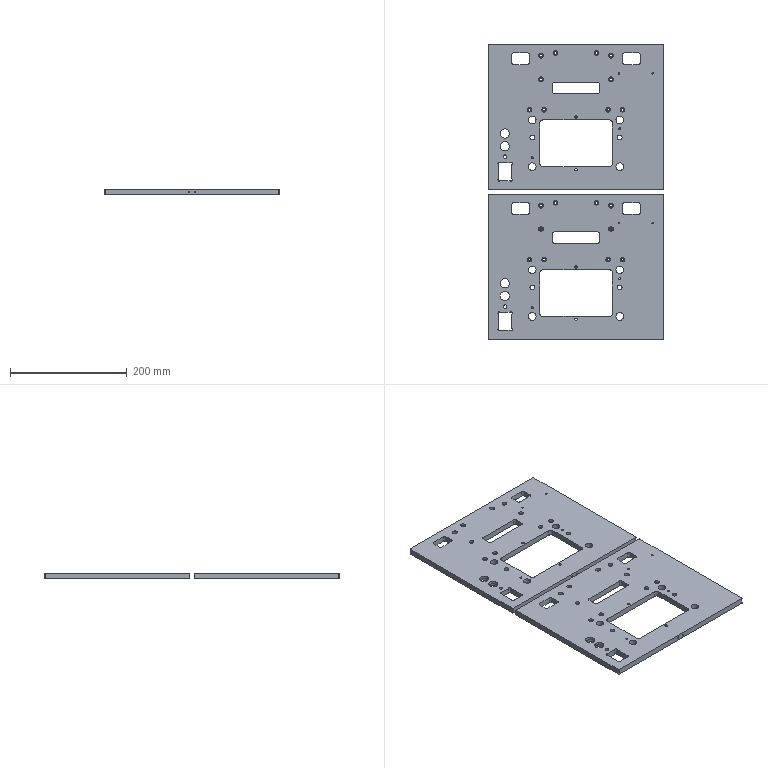NC program | NX | posted with a generic post | part box 300 x 507 x 10 mm
Whole program:
N10 G17 G21 G94 G90
(ZLEVEL_PROFILE_1_COPY_1_COPY_COPY , TOOL : D4A45)
N12 T02 M6
N14 G54
N16 G17 G0 G90 X44.225 Y79.686 S9500 M3
N18 G43 Z30. H2
N20 Z0.
N22 G94 G1 Z-1. F1000.
N24 X43.846 Y80.341
N26 G3 X43.5 Y80.541 R0.4
N28 X37.959 Y75. R5.541
N30 X43.5 Y80.541 R-5.541
N32 X43.154 Y80.341 R0.4
N34 G1 X42.775 Y79.686
N36 Z0.
N38 G0 Z30.
N40 X38.592 Y0.223
N42 Z0.
N44 G1 Z-1.
N46 X38.846 Y0.841
N48 G3 X38.5 Y1.041 R0.4
N50 X37.459 Y0. R1.041
N52 X38.5 Y1.041 R-1.041
N54 X38.154 Y0.841 R0.4
N56 G1 X38.408 Y0.223
N58 Z0.
N60 G0 Z30.
N62 X203.5 Y-131.791
N64 Z1.
N66 G1 Z-1.
N68 G3 X203.791 Y-131.5 R0.291
N70 X203.5 Y-131.791 R-0.291
N72 X203.673 Y-131.691 R0.2
N74 G1 Z0.
N76 G0 Z30.
N78 X48.178 Y131.357
N80 Z0.
N82 G1 Z-1.
N84 X47.898 Y131.841
N86 G3 X47.551 Y132.041 R0.4
N88 G1 X22.449
N90 G2 X21.694 Y132.41 R0.966
N92 G3 X20.094 Y130.803 R-1.141
N94 G2 X20.459 Y130.051 R0.956
N96 G1 Y112.949
N98 G2 X20.09 Y112.193 R0.967
N100 G3 X21.697 Y110.594 R-1.141
N102 G2 X22.449 Y110.959 R0.957
N104 G1 X47.551
N106 G2 X48.308 Y110.588 R0.97
N108 G3 X49.906 Y112.197 R-1.141
N110 G2 X49.541 Y112.949 R0.956
N112 G1 Y130.051
N114 G2 X49.911 Y130.807 R0.968
N116 G3 X48.303 Y132.406 R-1.141
N118 G2 X47.551 Y132.041 R0.957
N120 G3 X47.205 Y131.842 R0.4
N122 G1 X46.858 Y131.241
N124 Z0.
N126 G0 Z30.
N128 X140.228 Y-57.354
N130 Z0.
N132 G1 Z-1.
N134 X140.654 Y-58.091
N136 G3 X141. Y-58.291 R0.4
N138 G1 X141.001
N140 G3 X144.041 Y-55.249 R3.041
N142 X141. Y-58.291 R-3.041
N144 X141.346 Y-58.091 R0.4
N146 G1 X141.772 Y-57.354
N148 Z0.
N150 G0 Z30.
N152 X140.228 Y-82.104
N154 Z0.
N156 G1 Z-1.
N158 X140.654 Y-82.841
N160 G3 X141. Y-83.041 R0.4
N162 G1 X141.001
N164 G3 X144.041 Y-79.999 R3.041
N166 X141. Y-83.041 R-3.041
N168 X141.346 Y-82.841 R0.4
N170 G1 X141.772 Y-82.104
N172 Z0.
N174 G0 Z30.
N176 Y56.854
N178 Z0.
N180 G1 Z-1.
N182 X141.346 Y57.591
N184 G3 X141. Y57.791 R0.4
N186 X137.959 Y54.75 R3.041
N188 X141. Y57.791 R-3.041
N190 X140.654 Y57.591 R0.4
N192 G1 X140.228 Y56.854
N194 Z0.
N196 G0 Z30.
N198 X141.772 Y82.104
N200 Z0.
N202 G1 Z-1.
N204 X141.346 Y82.841
N206 G3 X141. Y83.041 R0.4
N208 X137.959 Y80. R3.041
N210 X141. Y83.041 R-3.041
N212 X140.654 Y82.841 R0.4
N214 G1 X140.228 Y82.104
N216 Z0.
N218 G0 Z30.
N220 X128.723 Y-0.092
N222 Z0.
N224 G1 Z-1.
N226 X129.341 Y-0.346
N228 G3 X129.541 Y0. R0.4
N230 X128.5 Y1.041 R1.041
N232 X129.541 Y0. R-1.041
N234 X129.341 Y0.346 R0.4
N236 G1 X128.723 Y0.092
N238 Z0.
N240 G0 Z30.
N242 X203.791 Y-73.5
N244 Z1.
N246 G1 Z-1.
N248 G3 X203.5 Y-73.209 R0.291
N250 X203.791 Y-73.5 R-0.291
N252 X203.691 Y-73.327 R0.2
N254 G1 Z0.
N256 G0 Z30.
N258 X235.604 Y-60.772
N260 Z0.
N262 G1 Z-1.
N264 X236.341 Y-60.346
N266 G3 X236.541 Y-60. R0.4
N268 X233.5 Y-56.959 R3.041
N270 X236.541 Y-60. R-3.041
N272 X236.341 Y-59.654 R0.4
N274 G1 X235.604 Y-59.228
N276 Z0.
N278 G0 Z30.
N280 X122.775 Y-79.686
N282 Z0.
N284 G1 Z-1.
N286 X123.154 Y-80.341
N288 G3 X123.5 Y-80.541 R0.4
N290 X129.041 Y-75. R5.541
N292 X123.5 Y-80.541 R-5.541
N294 X123.846 Y-80.341 R0.4
N296 G1 X124.225 Y-79.686
N298 Z0.
N300 G0 Z30.
N302 Y79.686
N304 Z0.
N306 G1 Z-1.
N308 X123.846 Y80.341
N310 G3 X123.5 Y80.541 R0.4
N312 G1 X123.496
N314 G3 X117.959 Y74.996 R5.541
N316 X123.5 Y80.541 R-5.541
N318 X123.154 Y80.341 R0.4
N320 G1 X122.775 Y79.686
N322 Z0.
N324 G0 Z30.
N326 X108.5 Y-75.691
N328 Z1.
N330 G1 Z-1.
N332 X108.501
N334 G3 X109.191 Y-74.999 R0.691
N336 X108.5 Y-75.691 R-0.691
N338 X108.846 Y-75.491 R0.4
N340 G1 Z0.
N342 G0 Z30.
N344 X235.604 Y59.228
N346 Z0.
N348 G1 Z-1.
N350 X236.341 Y59.654
N352 G3 X236.541 Y60. R0.4
N354 X233.5 Y63.041 R3.041
N356 X236.541 Y60. R-3.041
N358 X236.341 Y60.346 R0.4
N360 G1 X235.604 Y60.772
N362 Z0.
N364 G0 Z30.
N366 X101.217 Y128.2
N368 Z0.
N370 G1 Z-1.
N372 X100.846 Y128.841
N374 G3 X100.5 Y129.041 R0.4
N376 X93.459 Y122. R7.041
N378 X100.5 Y129.041 R-7.041
N380 X100.154 Y128.841 R0.4
N382 G1 X99.783 Y128.2
N384 Z0.
N386 G0 Z30.
N388 X195.604 Y-60.772
N390 Z0.
N392 G1 Z-1.
N394 X196.341 Y-60.346
N396 G3 X196.541 Y-60. R0.4
N398 X193.5 Y-56.959 R3.041
N400 X196.541 Y-60. R-3.041
N402 X196.341 Y-59.654 R0.4
N404 G1 X195.604 Y-59.228
N406 Z0.
N408 G0 Z30.
N410 Y59.228
N412 Z0.
N414 G1 Z-1.
N416 X196.341 Y59.654
N418 G3 X196.541 Y60. R0.4
N420 X193.5 Y63.041 R3.041
N422 X196.541 Y60. R-3.041
N424 X196.341 Y60.346 R0.4
N426 G1 X195.604 Y60.772
N428 Z0.
N430 G0 Z30.
N432 X94.272 Y77.104
N434 Z0.
N436 G1 Z-1.
N438 X93.846 Y77.841
N440 G3 X93.5 Y78.041 R0.4
N442 G1 X93.495
N444 G3 X90.459 Y74.995 R3.041
N446 X93.5 Y78.041 R-3.041
N448 X93.154 Y77.841 R0.4
N450 G1 X92.728 Y77.104
N452 Z0.
N454 G0 Z30.
N456 Y-77.104
N458 Z0.
N460 G1 Z-1.
N462 X93.154 Y-77.841
N464 G3 X93.5 Y-78.041 R0.4
N466 X96.541 Y-75. R3.041
N468 X93.5 Y-78.041 R-3.041
N470 X93.846 Y-77.841 R0.4
N472 G1 X94.272 Y-77.104
N474 Z0.
N476 G0 Z30.
N478 X240.604 Y-35.772
N480 Z0.
N482 G1 Z-1.
N484 X241.341 Y-35.346
N486 G3 X241.541 Y-35. R0.4
N488 X238.5 Y-31.959 R3.041
N490 X241.541 Y-35. R-3.041
N492 X241.341 Y-34.654 R0.4
N494 G1 X240.604 Y-34.228
N496 Z0.
N498 G0 Z30.
N500 X79.217 Y128.2
N502 Z0.
N504 G1 Z-1.
N506 X78.846 Y128.841
N508 G3 X78.5 Y129.041 R0.4
N510 X71.459 Y122. R7.041
N512 X78.5 Y129.041 R-7.041
N514 X78.154 Y128.841 R0.4
N516 G1 X77.783 Y128.2
N518 Z0.
N520 G0 Z30.
N522 X186.306 Y-37.944
N524 Z0.
N526 G1 Z-1.
N528 X187.341 Y-37.346
N530 G3 X187.541 Y-37. R0.4
N532 G1 Y37.
N534 G3 X185.5 Y39.041 R2.041
N536 G1 X171.5
N538 G3 X169.459 Y37. R2.041
N540 G1 Y-37.
N542 G3 X171.5 Y-39.041 R2.041
N544 G1 X185.5
N546 G3 X187.541 Y-37. R2.041
N548 X187.341 Y-36.654 R0.4
N550 G1 X186.741 Y-36.307
N552 Z0.
N554 G0 Z30.
N556 X61.444 Y122.306
N558 Z0.
N560 G1 Z-1.
N562 X60.846 Y123.341
N564 G3 X60.5 Y123.541 R0.4
N566 G1 X60.495
N568 G3 X58.459 Y121.495 R2.041
N570 X60.5 Y123.541 R-2.041
N572 X60.154 Y123.341 R0.4
N574 G1 X59.556 Y122.306
N576 Z0.
N578 G0 Z30.
N580 X58.5 Y75.691
N582 Z1.
N584 G1 Z-1.
N586 G3 X57.809 Y75. R0.691
N588 X58.5 Y75.691 R-0.691
N590 X58.154 Y75.491 R0.4
N592 G1 Z0.
N594 G0 Z30.
N596 X240.604 Y34.228
N598 Z0.
N600 G1 Z-1.
N602 X241.341 Y34.654
N604 G3 X241.541 Y35. R0.4
N606 X238.5 Y38.041 R3.041
N608 X241.541 Y35. R-3.041
N610 X241.341 Y35.346 R0.4
N612 G1 X240.604 Y35.772
N614 Z0.
N616 G0 Z30.
N618 X121.655 Y-58.243
N620 Z0.
N622 G1 Z-1.
N624 X122.341 Y-57.846
N626 G3 X122.541 Y-57.5 R0.4
N628 G1 Y57.
N630 G3 X118.5 Y61.041 R4.041
N632 G1 X48.5
N634 G3 X44.459 Y57. R4.041
N636 G1 Y-57.5
N638 G3 X48.5 Y-61.541 R4.041
N640 G1 X118.5
N642 G3 X122.541 Y-57.5 R4.041
N644 X122.341 Y-57.154 R0.4
N646 G1 X121.741 Y-56.807
N648 Z0.
N650 G0 Z30.
N652 X236.306 Y-107.944
N654 Z0.
N656 G1 Z-1.
N658 X237.341 Y-107.346
N660 G3 X237.541 Y-107. R0.4
N662 G1 Y-83.
N664 G3 X235.5 Y-80.959 R2.041
N666 G1 X221.5
N668 G3 X219.459 Y-83. R2.041
N670 G1 Y-107.
N672 G3 X221.5 Y-109.041 R2.041
N674 G1 X235.5
N676 G3 X237.541 Y-107. R2.041
N678 X237.341 Y-106.654 R0.4
N680 G1 X236.741 Y-106.307
N682 Z0.
N684 G0 Z30.
N686 X236.306 Y82.056
N688 Z0.
N690 G1 Z-1.
N692 X237.341 Y82.654
N694 G3 X237.541 Y83. R0.4
N696 G1 Y107.
N698 G3 X235.5 Y109.041 R2.041
N700 G1 X221.5
N702 G3 X219.459 Y107. R2.041
N704 G1 Y83.
N706 G3 X221.5 Y80.959 R2.041
N708 G1 X235.5
N710 G3 X237.541 Y83. R2.041
N712 X237.341 Y83.346 R0.4
N714 G1 X236.741 Y83.693
N716 Z0.
N718 G0 Z30.
N720 X42.775 Y-79.686
N722 Z0.
N724 G1 Z-1.
N726 X43.154 Y-80.341
N728 G3 X43.5 Y-80.541 R0.4
N730 G1 X43.502
N732 G3 X49.041 Y-74.998 R5.541
N734 X43.5 Y-80.541 R-5.541
N736 X43.846 Y-80.341 R0.4
N738 G1 X44.225 Y-79.686
N740 Z0.
N742 G0 Z30.
N744 X-17.728 Y37.104
N746 Z0.
N748 G1 Z-1.
N750 X-18.154 Y37.841
N752 G3 X-18.5 Y38.041 R0.4
N754 X-21.541 Y35. R3.041
N756 X-18.5 Y38.041 R-3.041
N758 X-18.846 Y37.841 R0.4
N760 G1 X-19.272 Y37.104
N762 Z0.
N764 G0 Z30.
N766 Y-37.104
N768 Z0.
N770 G1 Z-1.
N772 X-18.846 Y-37.841
N774 G3 X-18.5 Y-38.041 R0.4
N776 X-15.459 Y-34.999 R3.041
N778 X-18.5 Y-38.041 R-3.041
N780 X-18.154 Y-37.841 R0.4
N782 G1 X-17.728 Y-37.104
N784 Z0.
N786 G0 Z30.
N788 X-24.272 Y-62.104
N790 Z0.
N792 G1 Z-1.
N794 X-23.846 Y-62.841
N796 G3 X-23.5 Y-63.041 R0.4
N798 G1 X-23.497
N800 G3 X-20.459 Y-59.997 R3.041
N802 X-23.5 Y-63.041 R-3.041
N804 X-23.154 Y-62.841 R0.4
N806 G1 X-22.728 Y-62.104
N808 Z0.
N810 G0 Z30.
N812 Y62.104
N814 Z0.
N816 G1 Z-1.
N818 X-23.154 Y62.841
N820 G3 X-23.5 Y63.041 R0.4
N822 X-26.541 Y60. R3.041
N824 X-23.5 Y63.041 R-3.041
N826 X-23.846 Y62.841 R0.4
N828 G1 X-24.272 Y62.104
N830 Z0.
N832 G0 Z30.
N834 X-20.694 Y-107.944
N836 Z0.
N838 G1 Z-1.
N840 X-19.659 Y-107.346
N842 G3 X-19.459 Y-107. R0.4
N844 G1 Y-83.
N846 G3 X-21.5 Y-80.959 R2.041
N848 G1 X-35.5
N850 G3 X-37.541 Y-83. R2.041
N852 G1 Y-107.
N854 G3 X-35.5 Y-109.041 R2.041
N856 G1 X-21.5
N858 G3 X-19.459 Y-107. R2.041
N860 X-19.659 Y-106.654 R0.4
N862 G1 X-20.259 Y-106.307
N864 Z0.
N866 G0 Z30.
N868 X-20.694 Y82.056
N870 Z0.
N872 G1 Z-1.
N874 X-19.659 Y82.654
N876 G3 X-19.459 Y83. R0.4
N878 G1 Y107.
N880 G3 X-21.5 Y109.041 R2.041
N882 G1 X-35.5
N884 G3 X-37.541 Y107. R2.041
N886 G1 Y83.
N888 G3 X-35.5 Y80.959 R2.041
N890 G1 X-21.5
N892 G3 X-19.459 Y83. R2.041
N894 X-19.659 Y83.346 R0.4
N896 G1 X-20.259 Y83.693
N898 Z0.
N900 G0 Z30.
N902 X-53.5 Y-131.791
N904 Z1.
N906 G1 Z-1.
N908 G3 X-53.209 Y-131.5 R0.291
N910 X-53.5 Y-131.791 R-0.291
N912 X-53.327 Y-131.691 R0.2
N914 G1 Z0.
N916 G0 Z30.
N918 X-53.5 Y-73.791
N920 Z1.
N922 G1 Z-1.
N924 G3 X-53.209 Y-73.5 R0.291
N926 X-53.5 Y-73.791 R-0.291
N928 X-53.327 Y-73.691 R0.2
N930 G1 Z0.
N932 G0 Z30.
N934 X-64.272 Y-62.104
N936 Z0.
N938 G1 Z-1.
N940 X-63.846 Y-62.841
N942 G3 X-63.5 Y-63.041 R0.4
N944 G1 X-63.494
N946 G3 X-60.459 Y-59.994 R3.041
N948 X-63.5 Y-63.041 R-3.041
N950 X-63.154 Y-62.841 R0.4
N952 G1 X-62.728 Y-62.104
N954 Z0.
N956 G0 Z30.
N958 Y62.104
N960 Z0.
N962 G1 Z-1.
N964 X-63.154 Y62.841
N966 G3 X-63.5 Y63.041 R0.4
N968 X-66.541 Y60. R3.041
N970 X-63.5 Y63.041 R-3.041
N972 X-63.846 Y62.841 R0.4
N974 G1 X-64.272 Y62.104
N976 Z0.
N978 G0 Z30.
N980 X-70.694 Y-37.944
N982 Z0.
N984 G1 Z-1.
N986 X-69.659 Y-37.346
N988 G3 X-69.459 Y-37. R0.4
N990 G1 Y37.
N992 G3 X-71.5 Y39.041 R2.041
N994 G1 X-85.5
N996 G3 X-87.541 Y37. R2.041
N998 G1 Y-37.
N1000 G3 X-85.5 Y-39.041 R2.041
N1002 G1 X-71.5
N1004 G3 X-69.459 Y-37. R2.041
N1006 X-69.659 Y-36.654 R0.4
N1008 G1 X-70.259 Y-36.307
N1010 Z0.
N1012 G0 Z30.
N1014 X-116.772 Y-82.104
N1016 Z0.
N1018 G1 Z-1.
N1020 X-116.346 Y-82.841
N1022 G3 X-116. Y-83.041 R0.4
N1024 G1 X-115.999
N1026 G3 X-112.959 Y-79.999 R3.041
N1028 X-116. Y-83.041 R-3.041
N1030 X-115.654 Y-82.841 R0.4
N1032 G1 X-115.228 Y-82.104
N1034 Z0.
N1036 G0 Z30.
N1038 X-116.772 Y-57.354
N1040 Z0.
N1042 G1 Z-1.
N1044 X-116.346 Y-58.091
N1046 G3 X-116. Y-58.291 R0.4
N1048 G1 X-115.999
N1050 G3 X-112.959 Y-55.249 R3.041
N1052 X-116. Y-58.291 R-3.041
N1054 X-115.654 Y-58.091 R0.4
N1056 G1 X-115.228 Y-57.354
N1058 Z0.
N1060 G0 Z30.
N1062 Y56.854
N1064 Z0.
N1066 G1 Z-1.
N1068 X-115.654 Y57.591
N1070 G3 X-116. Y57.791 R0.4
N1072 X-119.041 Y54.75 R3.041
N1074 X-116. Y57.791 R-3.041
N1076 X-116.346 Y57.591 R0.4
N1078 G1 X-116.772 Y56.854
N1080 Z0.
N1082 G0 Z30.
N1084 X-115.228 Y82.104
N1086 Z0.
N1088 G1 Z-1.
N1090 X-115.654 Y82.841
N1092 G3 X-116. Y83.041 R0.4
N1094 X-119.041 Y80. R3.041
N1096 X-116. Y83.041 R-3.041
N1098 X-116.346 Y82.841 R0.4
N1100 G1 X-116.772 Y82.104
N1102 Z0.
N1104 G0 Z30.
N1106 X-128.723 Y0.092
N1108 Z0.
N1110 G1 Z-1.
N1112 X-129.341 Y0.346
N1114 G3 X-129.541 Y0. R0.4
N1116 X-128.5 Y-1.041 R1.041
N1118 X-129.541 Y0. R-1.041
N1120 X-129.341 Y-0.346 R0.4
N1122 G1 X-128.723 Y-0.092
N1124 Z0.
N1126 G0 Z30.
N1128 X-132.775 Y79.686
N1130 Z0.
N1132 G1 Z-1.
N1134 X-133.154 Y80.341
N1136 G3 X-133.5 Y80.541 R0.4
N1138 G1 X-133.504
N1140 G3 X-139.041 Y74.996 R5.541
N1142 X-133.5 Y80.541 R-5.541
N1144 X-133.846 Y80.341 R0.4
N1146 G1 X-134.225 Y79.686
N1148 Z0.
N1150 G0 Z30.
N1152 Y-79.686
N1154 Z0.
N1156 G1 Z-1.
N1158 X-133.846 Y-80.341
N1160 G3 X-133.5 Y-80.541 R0.4
N1162 X-127.959 Y-75. R5.541
N1164 X-133.5 Y-80.541 R-5.541
N1166 X-133.154 Y-80.341 R0.4
N1168 G1 X-132.775 Y-79.686
N1170 Z0.
N1172 G0 Z30.
N1174 X-148.5 Y-75.691
N1176 Z1.
N1178 G1 Z-1.
N1180 X-148.498
N1182 G3 X-147.809 Y-74.998 R0.691
N1184 X-148.5 Y-75.691 R-0.691
N1186 X-148.154 Y-75.491 R0.4
N1188 G1 Z0.
N1190 G0 Z30.
N1192 X-155.783 Y128.2
N1194 Z0.
N1196 G1 Z-1.
N1198 X-156.154 Y128.841
N1200 G3 X-156.5 Y129.041 R0.4
N1202 X-163.541 Y122. R7.041
N1204 X-156.5 Y129.041 R-7.041
N1206 X-156.846 Y128.841 R0.4
N1208 G1 X-157.217 Y128.2
N1210 Z0.
N1212 G0 Z30.
N1214 X-164.272 Y-77.104
N1216 Z0.
N1218 G1 Z-1.
N1220 X-163.846 Y-77.841
N1222 G3 X-163.5 Y-78.041 R0.4
N1224 X-160.459 Y-75. R3.041
N1226 X-163.5 Y-78.041 R-3.041
N1228 X-163.154 Y-77.841 R0.4
N1230 G1 X-162.728 Y-77.104
N1232 Z0.
N1234 G0 Z30.
N1236 Y77.104
N1238 Z0.
N1240 G1 Z-1.
N1242 X-163.154 Y77.841
N1244 G3 X-163.5 Y78.041 R0.4
N1246 G1 X-163.505
N1248 G3 X-166.541 Y74.995 R3.041
N1250 X-163.5 Y78.041 R-3.041
N1252 X-163.846 Y77.841 R0.4
N1254 G1 X-164.272 Y77.104
N1256 Z0.
N1258 G0 Z30.
N1260 X-177.783 Y128.2
N1262 Z0.
N1264 G1 Z-1.
N1266 X-178.154 Y128.841
N1268 G3 X-178.5 Y129.041 R0.4
N1270 X-185.541 Y122. R7.041
N1272 X-178.5 Y129.041 R-7.041
N1274 X-178.846 Y128.841 R0.4
N1276 G1 X-179.217 Y128.2
N1278 Z0.
N1280 G0 Z30.
N1282 X-195.556 Y122.306
N1284 Z0.
N1286 G1 Z-1.
N1288 X-196.154 Y123.341
N1290 G3 X-196.5 Y123.541 R0.4
N1292 G1 X-196.505
N1294 G3 X-198.541 Y121.495 R2.041
N1296 X-196.5 Y123.541 R-2.041
N1298 X-196.846 Y123.341 R0.4
N1300 G1 X-197.444 Y122.306
N1302 Z0.
N1304 G0 Z30.
N1306 X-199.191 Y75.
N1308 Z1.
N1310 G1 Z-1.
N1312 G3 X-198.5 Y74.309 R0.691
N1314 X-199.191 Y75. R-0.691
N1316 X-198.991 Y74.654 R0.4
N1318 G1 Z0.
N1320 G0 Z30.
N1322 X-211.655 Y57.743
N1324 Z0.
N1326 G1 Z-1.
N1328 X-212.341 Y57.346
N1330 G3 X-212.541 Y57. R0.4
N1332 G1 Y-57.5
N1334 G3 X-208.5 Y-61.541 R4.041
N1336 G1 X-138.5
N1338 G3 X-134.459 Y-57.5 R4.041
N1340 G1 Y57.
N1342 G3 X-138.5 Y61.041 R4.041
N1344 G1 X-208.5
N1346 G3 X-212.541 Y57. R4.041
N1348 X-212.341 Y56.654 R0.4
N1350 G1 X-211.741 Y56.307
N1352 Z0.
N1354 G0 Z30.
N1356 X-218.186 Y-74.275
N1358 Z0.
N1360 G1 Z-1.
N1362 X-218.841 Y-74.654
N1364 G3 X-219.041 Y-75. R0.4
N1366 X-213.5 Y-80.541 R5.541
N1368 X-219.041 Y-75. R-5.541
N1370 X-218.841 Y-75.346 R0.4
N1372 G1 X-218.186 Y-75.725
N1374 Z0.
N1376 G0 Z30.
N1378 Y75.725
N1380 Z0.
N1382 G1 Z-1.
N1384 X-218.841 Y75.346
N1386 G3 X-219.041 Y75. R0.4
N1388 X-213.5 Y69.459 R5.541
N1390 X-219.041 Y75. R-5.541
N1392 X-218.841 Y74.654 R0.4
N1394 G1 X-218.186 Y74.275
N1396 Z0.
N1398 G0 Z30.
N1400 X-218.723 Y0.092
N1402 Z0.
N1404 G1 Z-1.
N1406 X-219.341 Y0.346
N1408 G3 X-219.541 Y0. R0.4
N1410 X-218.5 Y-1.041 R1.041
N1412 X-219.541 Y0. R-1.041
N1414 X-219.341 Y-0.346 R0.4
N1416 G1 X-218.723 Y-0.092
N1418 Z0.
N1420 G0 Z30.
N1422 X-208.822 Y131.357
N1424 Z0.
N1426 G1 Z-1.
N1428 X-209.102 Y131.841
N1430 G3 X-209.448 Y132.041 R0.4
N1432 G1 X-234.552
N1434 G2 X-235.307 Y132.41 R0.967
N1436 G3 X-236.906 Y130.803 R-1.141
N1438 G2 X-236.541 Y130.051 R0.957
N1440 G1 Y112.949
N1442 G2 X-236.908 Y112.196 R0.96
N1444 G3 X-235.303 Y110.594 R-1.141
N1446 G2 X-234.552 Y110.959 R0.956
N1448 G1 X-209.448
N1450 G2 X-208.693 Y110.59 R0.967
N1452 G3 X-207.094 Y112.197 R-1.141
N1454 G2 X-207.459 Y112.949 R0.956
N1456 G1 Y130.051
N1458 G2 X-207.09 Y130.807 R0.967
N1460 G3 X-208.697 Y132.406 R-1.141
N1462 G2 X-209.448 Y132.041 R0.956
N1464 G3 X-209.795 Y131.842 R0.4
N1466 G1 X-210.142 Y131.241
N1468 Z0.
N1470 G0 Z30.
N1472 X-255.192 Y-149.154
N1474 Z0.
N1476 G1 Z-1.
N1478 X-254.659 Y-148.846
N1480 G3 X-254.459 Y-148.5 R0.4
N1482 G1 Y148.5
N1484 G2 X-252. Y150.959 R2.459
N1486 G1 X-5.
N1488 G2 X-2.541 Y148.5 R2.459
N1490 G1 Y-148.5
N1492 G2 X-5. Y-150.959 R2.459
N1494 G1 X-252.
N1496 G2 X-254.459 Y-148.5 R2.459
N1498 G3 X-254.659 Y-148.154 R0.4
N1500 G1 X-255.259 Y-147.807
N1502 Z0.
N1504 G0 Z30.
N1506 X255.192 Y149.154
N1508 Z0.
N1510 G1 Z-1.
N1512 X254.659 Y148.846
N1514 G3 X254.459 Y148.5 R0.4
N1516 G1 Y-148.5
N1518 G2 X252. Y-150.959 R2.459
N1520 G1 X5.
N1522 G2 X2.541 Y-148.5 R2.459
N1524 G1 Y148.5
N1526 G2 X5. Y150.959 R2.459
N1528 G1 X252.
N1530 G2 X254.459 Y148.5 R2.459
N1532 G3 X254.659 Y148.154 R0.4
N1534 G1 X255.259 Y147.807
N1536 Z0.
N1538 G0 Z30.
N1540 M5
(ZLEVEL_PROFILE_COPY_COPY_1_COPY , TOOL : D6)
N1542 T06 M6
N1544 G54
N1546 G17 G0 G90 X-256.6 Y-37.876 S9500 M3
N1548 G43 Z30. H6
N1550 Z1.5
N1552 G94 G1 Y0. Z-0.485 F1000.
N1554 Y148.5 F2200.
N1556 G2 X-252. Y153.1 R4.6
N1558 G1 X-5.
N1560 G2 X-0.4 Y148.5 R4.6
N1562 G1 Y-148.5
N1564 G2 X-5. Y-153.1 R4.6
N1566 G1 X-252.
N1568 G2 X-256.6 Y-148.5 R4.6
N1570 G1 Y0.
N1572 Y27.786 Z-0.97
N1574 Y148.5
N1576 G2 X-252. Y153.1 R4.6
N1578 G1 X-5.
N1580 G2 X-0.4 Y148.5 R4.6
N1582 G1 Y-148.5
N1584 G2 X-5. Y-153.1 R4.6
N1586 G1 X-252.
N1588 G2 X-256.6 Y-148.5 R4.6
N1590 G1 Y0.
N1592 Y27.786 Z-1.455
N1594 Y148.5
N1596 G2 X-252. Y153.1 R4.6
N1598 G1 X-5.
N1600 G2 X-0.4 Y148.5 R4.6
N1602 G1 Y-148.5
N1604 G2 X-5. Y-153.1 R4.6
N1606 G1 X-252.
N1608 G2 X-256.6 Y-148.5 R4.6
N1610 G1 Y0.
N1612 Y27.786 Z-1.94
N1614 Y148.5
N1616 G2 X-252. Y153.1 R4.6
N1618 G1 X-5.
N1620 G2 X-0.4 Y148.5 R4.6
N1622 G1 Y-148.5
N1624 G2 X-5. Y-153.1 R4.6
N1626 G1 X-252.
N1628 G2 X-256.6 Y-148.5 R4.6
N1630 G1 Y0.
N1632 Y27.786 Z-2.425
N1634 Y148.5
N1636 G2 X-252. Y153.1 R4.6
N1638 G1 X-5.
N1640 G2 X-0.4 Y148.5 R4.6
N1642 G1 Y-148.5
N1644 G2 X-5. Y-153.1 R4.6
N1646 G1 X-252.
N1648 G2 X-256.6 Y-148.5 R4.6
N1650 G1 Y0.
N1652 Y27.786 Z-2.91
N1654 Y148.5
N1656 G2 X-252. Y153.1 R4.6
N1658 G1 X-5.
N1660 G2 X-0.4 Y148.5 R4.6
N1662 G1 Y-148.5
N1664 G2 X-5. Y-153.1 R4.6
N1666 G1 X-252.
N1668 G2 X-256.6 Y-148.5 R4.6
N1670 G1 Y0.
N1672 Y27.786 Z-3.395
N1674 Y148.5
N1676 G2 X-252. Y153.1 R4.6
N1678 G1 X-5.
N1680 G2 X-0.4 Y148.5 R4.6
N1682 G1 Y-148.5
N1684 G2 X-5. Y-153.1 R4.6
N1686 G1 X-252.
N1688 G2 X-256.6 Y-148.5 R4.6
N1690 G1 Y0.
N1692 Y27.786 Z-3.88
N1694 Y148.5
N1696 G2 X-252. Y153.1 R4.6
N1698 G1 X-5.
N1700 G2 X-0.4 Y148.5 R4.6
N1702 G1 Y-148.5
N1704 G2 X-5. Y-153.1 R4.6
N1706 G1 X-252.
N1708 G2 X-256.6 Y-148.5 R4.6
N1710 G1 Y0.
N1712 Y27.786 Z-4.365
N1714 Y148.5
N1716 G2 X-252. Y153.1 R4.6
N1718 G1 X-5.
N1720 G2 X-0.4 Y148.5 R4.6
N1722 G1 Y-148.5
N1724 G2 X-5. Y-153.1 R4.6
N1726 G1 X-252.
N1728 G2 X-256.6 Y-148.5 R4.6
N1730 G1 Y0.
N1732 Y27.786 Z-4.85
N1734 Y148.5
N1736 G2 X-252. Y153.1 R4.6
N1738 G1 X-5.
N1740 G2 X-0.4 Y148.5 R4.6
N1742 G1 Y-148.5
N1744 G2 X-5. Y-153.1 R4.6
N1746 G1 X-252.
N1748 G2 X-256.6 Y-148.5 R4.6
N1750 G1 Y0.
N1752 Y27.786 Z-5.335
N1754 Y148.5
N1756 G2 X-252. Y153.1 R4.6
N1758 G1 X-5.
N1760 G2 X-0.4 Y148.5 R4.6
N1762 G1 Y-148.5
N1764 G2 X-5. Y-153.1 R4.6
N1766 G1 X-252.
N1768 G2 X-256.6 Y-148.5 R4.6
N1770 G1 Y0.
N1772 Y27.786 Z-5.82
N1774 Y148.5
N1776 G2 X-252. Y153.1 R4.6
N1778 G1 X-5.
N1780 G2 X-0.4 Y148.5 R4.6
N1782 G1 Y-148.5
N1784 G2 X-5. Y-153.1 R4.6
N1786 G1 X-252.
N1788 G2 X-256.6 Y-148.5 R4.6
N1790 G1 Y0.
N1792 Y27.786 Z-6.305
N1794 Y148.5
N1796 G2 X-252. Y153.1 R4.6
N1798 G1 X-5.
N1800 G2 X-0.4 Y148.5 R4.6
N1802 G1 Y-148.5
N1804 G2 X-5. Y-153.1 R4.6
N1806 G1 X-252.
N1808 G2 X-256.6 Y-148.5 R4.6
N1810 G1 Y0.
N1812 Y27.786 Z-6.79
N1814 Y148.5
N1816 G2 X-252. Y153.1 R4.6
N1818 G1 X-5.
N1820 G2 X-0.4 Y148.5 R4.6
N1822 G1 Y-148.5
N1824 G2 X-5. Y-153.1 R4.6
N1826 G1 X-252.
N1828 G2 X-256.6 Y-148.5 R4.6
N1830 G1 Y0.
N1832 Y27.786 Z-7.275
N1834 Y148.5
N1836 G2 X-252. Y153.1 R4.6
N1838 G1 X-5.
N1840 G2 X-0.4 Y148.5 R4.6
N1842 G1 Y-148.5
N1844 G2 X-5. Y-153.1 R4.6
N1846 G1 X-252.
N1848 G2 X-256.6 Y-148.5 R4.6
N1850 G1 Y0.
N1852 Y27.786 Z-7.76
N1854 Y148.5
N1856 G2 X-252. Y153.1 R4.6
N1858 G1 X-5.
N1860 G2 X-0.4 Y148.5 R4.6
N1862 G1 Y-148.5
N1864 G2 X-5. Y-153.1 R4.6
N1866 G1 X-252.
N1868 G2 X-256.6 Y-148.5 R4.6
N1870 G1 Y0.
N1872 Y27.786 Z-8.245
N1874 Y148.5
N1876 G2 X-252. Y153.1 R4.6
N1878 G1 X-5.
N1880 G2 X-0.4 Y148.5 R4.6
N1882 G1 Y-148.5
N1884 G2 X-5. Y-153.1 R4.6
N1886 G1 X-252.
N1888 G2 X-256.6 Y-148.5 R4.6
N1890 G1 Y0.
N1892 Y27.786 Z-8.73
N1894 Y148.5
N1896 G2 X-252. Y153.1 R4.6
N1898 G1 X-5.
N1900 G2 X-0.4 Y148.5 R4.6
N1902 G1 Y-148.5
N1904 G2 X-5. Y-153.1 R4.6
N1906 G1 X-252.
N1908 G2 X-256.6 Y-148.5 R4.6
N1910 G1 Y0.
N1912 Y27.786 Z-9.215
N1914 Y148.5
N1916 G2 X-252. Y153.1 R4.6
N1918 G1 X-5.
N1920 G2 X-0.4 Y148.5 R4.6
N1922 G1 Y-148.5
N1924 G2 X-5. Y-153.1 R4.6
N1926 G1 X-252.
N1928 G2 X-256.6 Y-148.5 R4.6
N1930 G1 Y0.
N1932 Y27.786 Z-9.7
N1934 Y148.5
N1936 G2 X-252. Y153.1 R4.6
N1938 G1 X-5.
N1940 G2 X-0.4 Y148.5 R4.6
N1942 G1 Y-148.5
N1944 G2 X-5. Y-153.1 R4.6
N1946 G1 X-252.
N1948 G2 X-256.6 Y-148.5 R4.6
N1950 G1 Y27.786
N1952 Z-8.2
N1954 G0 Z30.
N1956 X256.6 Y37.876
N1958 Z1.5
N1960 G1 Y0. Z-0.485 F1000.
N1962 Y-148.5 F2200.
N1964 G2 X252. Y-153.1 R4.6
N1966 G1 X5.
N1968 G2 X0.4 Y-148.5 R4.6
N1970 G1 Y148.5
N1972 G2 X5. Y153.1 R4.6
N1974 G1 X252.
N1976 G2 X256.6 Y148.5 R4.6
N1978 G1 Y0.
N1980 Y-27.786 Z-0.97
N1982 Y-148.5
N1984 G2 X252. Y-153.1 R4.6
N1986 G1 X5.
N1988 G2 X0.4 Y-148.5 R4.6
N1990 G1 Y148.5
N1992 G2 X5. Y153.1 R4.6
N1994 G1 X252.
N1996 G2 X256.6 Y148.5 R4.6
N1998 G1 Y0.
N2000 Y-27.786 Z-1.455
N2002 Y-148.5
N2004 G2 X252. Y-153.1 R4.6
N2006 G1 X5.
N2008 G2 X0.4 Y-148.5 R4.6
N2010 G1 Y148.5
N2012 G2 X5. Y153.1 R4.6
N2014 G1 X252.
N2016 G2 X256.6 Y148.5 R4.6
N2018 G1 Y0.
N2020 Y-27.786 Z-1.94
N2022 Y-148.5
N2024 G2 X252. Y-153.1 R4.6
N2026 G1 X5.
N2028 G2 X0.4 Y-148.5 R4.6
N2030 G1 Y148.5
N2032 G2 X5. Y153.1 R4.6
N2034 G1 X252.
N2036 G2 X256.6 Y148.5 R4.6
N2038 G1 Y0.
N2040 Y-27.786 Z-2.425
N2042 Y-148.5
N2044 G2 X252. Y-153.1 R4.6
N2046 G1 X5.
N2048 G2 X0.4 Y-148.5 R4.6
N2050 G1 Y148.5
N2052 G2 X5. Y153.1 R4.6
N2054 G1 X252.
N2056 G2 X256.6 Y148.5 R4.6
N2058 G1 Y0.
N2060 Y-27.786 Z-2.91
N2062 Y-148.5
N2064 G2 X252. Y-153.1 R4.6
N2066 G1 X5.
N2068 G2 X0.4 Y-148.5 R4.6
N2070 G1 Y148.5
N2072 G2 X5. Y153.1 R4.6
N2074 G1 X252.
N2076 G2 X256.6 Y148.5 R4.6
N2078 G1 Y0.
N2080 Y-27.786 Z-3.395
N2082 Y-148.5
N2084 G2 X252. Y-153.1 R4.6
N2086 G1 X5.
N2088 G2 X0.4 Y-148.5 R4.6
N2090 G1 Y148.5
N2092 G2 X5. Y153.1 R4.6
N2094 G1 X252.
N2096 G2 X256.6 Y148.5 R4.6
N2098 G1 Y0.
N2100 Y-27.786 Z-3.88
N2102 Y-148.5
N2104 G2 X252. Y-153.1 R4.6
N2106 G1 X5.
N2108 G2 X0.4 Y-148.5 R4.6
N2110 G1 Y148.5
N2112 G2 X5. Y153.1 R4.6
N2114 G1 X252.
N2116 G2 X256.6 Y148.5 R4.6
N2118 G1 Y0.
N2120 Y-27.786 Z-4.365
N2122 Y-148.5
N2124 G2 X252. Y-153.1 R4.6
N2126 G1 X5.
N2128 G2 X0.4 Y-148.5 R4.6
N2130 G1 Y148.5
N2132 G2 X5. Y153.1 R4.6
N2134 G1 X252.
N2136 G2 X256.6 Y148.5 R4.6
N2138 G1 Y0.
N2140 Y-27.786 Z-4.85
N2142 Y-148.5
N2144 G2 X252. Y-153.1 R4.6
N2146 G1 X5.
N2148 G2 X0.4 Y-148.5 R4.6
N2150 G1 Y148.5
N2152 G2 X5. Y153.1 R4.6
N2154 G1 X252.
N2156 G2 X256.6 Y148.5 R4.6
N2158 G1 Y0.
N2160 Y-27.786 Z-5.335
N2162 Y-148.5
N2164 G2 X252. Y-153.1 R4.6
N2166 G1 X5.
N2168 G2 X0.4 Y-148.5 R4.6
N2170 G1 Y148.5
N2172 G2 X5. Y153.1 R4.6
N2174 G1 X252.
N2176 G2 X256.6 Y148.5 R4.6
N2178 G1 Y0.
N2180 Y-27.786 Z-5.82
N2182 Y-148.5
N2184 G2 X252. Y-153.1 R4.6
N2186 G1 X5.
N2188 G2 X0.4 Y-148.5 R4.6
N2190 G1 Y148.5
N2192 G2 X5. Y153.1 R4.6
N2194 G1 X252.
N2196 G2 X256.6 Y148.5 R4.6
N2198 G1 Y0.
N2200 Y-27.786 Z-6.305
N2202 Y-148.5
N2204 G2 X252. Y-153.1 R4.6
N2206 G1 X5.
N2208 G2 X0.4 Y-148.5 R4.6
N2210 G1 Y148.5
N2212 G2 X5. Y153.1 R4.6
N2214 G1 X252.
N2216 G2 X256.6 Y148.5 R4.6
N2218 G1 Y0.
N2220 Y-27.786 Z-6.79
N2222 Y-148.5
N2224 G2 X252. Y-153.1 R4.6
N2226 G1 X5.
N2228 G2 X0.4 Y-148.5 R4.6
N2230 G1 Y148.5
N2232 G2 X5. Y153.1 R4.6
N2234 G1 X252.
N2236 G2 X256.6 Y148.5 R4.6
N2238 G1 Y0.
N2240 Y-27.786 Z-7.275
N2242 Y-148.5
N2244 G2 X252. Y-153.1 R4.6
N2246 G1 X5.
N2248 G2 X0.4 Y-148.5 R4.6
N2250 G1 Y148.5
N2252 G2 X5. Y153.1 R4.6
N2254 G1 X252.
N2256 G2 X256.6 Y148.5 R4.6
N2258 G1 Y0.
N2260 Y-27.786 Z-7.76
N2262 Y-148.5
N2264 G2 X252. Y-153.1 R4.6
N2266 G1 X5.
N2268 G2 X0.4 Y-148.5 R4.6
N2270 G1 Y148.5
N2272 G2 X5. Y153.1 R4.6
N2274 G1 X252.
N2276 G2 X256.6 Y148.5 R4.6
N2278 G1 Y0.
N2280 Y-27.786 Z-8.245
N2282 Y-148.5
N2284 G2 X252. Y-153.1 R4.6
N2286 G1 X5.
N2288 G2 X0.4 Y-148.5 R4.6
N2290 G1 Y148.5
N2292 G2 X5. Y153.1 R4.6
N2294 G1 X252.
N2296 G2 X256.6 Y148.5 R4.6
N2298 G1 Y0.
N2300 Y-27.786 Z-8.73
N2302 Y-148.5
N2304 G2 X252. Y-153.1 R4.6
N2306 G1 X5.
N2308 G2 X0.4 Y-148.5 R4.6
N2310 G1 Y148.5
N2312 G2 X5. Y153.1 R4.6
N2314 G1 X252.
N2316 G2 X256.6 Y148.5 R4.6
N2318 G1 Y0.
N2320 Y-27.786 Z-9.215
N2322 Y-148.5
N2324 G2 X252. Y-153.1 R4.6
N2326 G1 X5.
N2328 G2 X0.4 Y-148.5 R4.6
N2330 G1 Y148.5
N2332 G2 X5. Y153.1 R4.6
N2334 G1 X252.
N2336 G2 X256.6 Y148.5 R4.6
N2338 G1 Y0.
N2340 Y-27.786 Z-9.7
N2342 Y-148.5
N2344 G2 X252. Y-153.1 R4.6
N2346 G1 X5.
N2348 G2 X0.4 Y-148.5 R4.6
N2350 G1 Y148.5
N2352 G2 X5. Y153.1 R4.6
N2354 G1 X252.
N2356 G2 X256.6 Y148.5 R4.6
N2358 G1 Y-27.786
N2360 Z-8.2
N2362 G0 Z30.
N2364 M5
N2366 M2